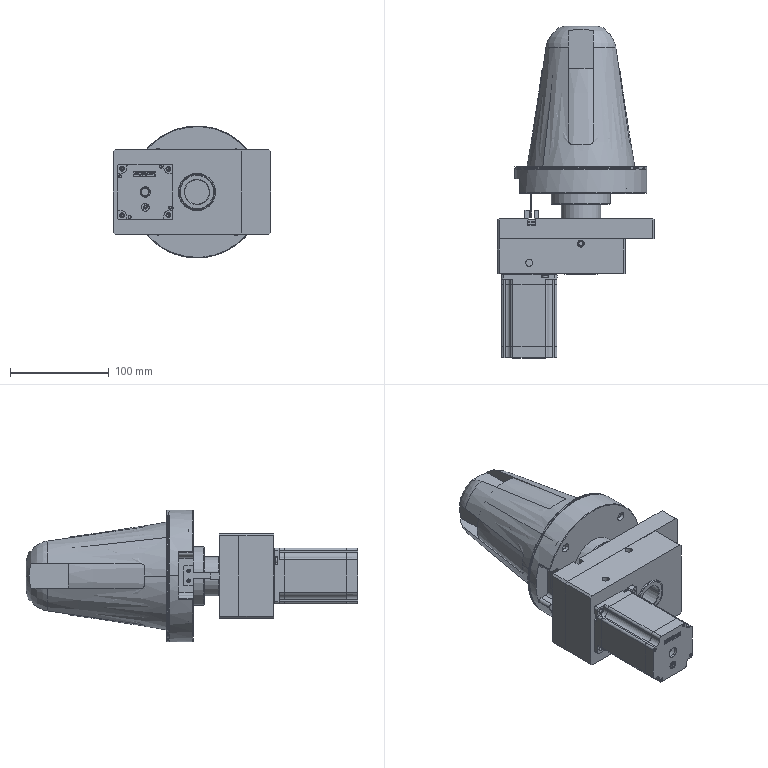Part | SolidWorks | 24 solids | 3052 faces | volume 1851782 mm3 | plane 1400 | cylinder 1094 | spline 313 | cone 243 | torus 2 | commonest cylinder face diameters 0.5 x256 72 x74 67.5 x71 0.6 x62 3 x42 32.5 x35